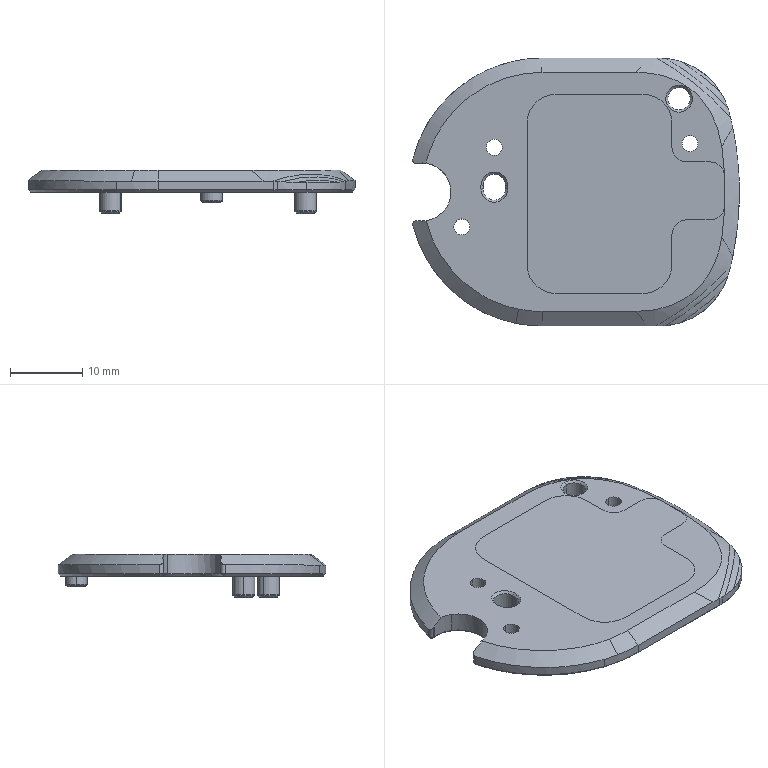NC program | NX | posted with a generic post | part box 45.101 x 36.973 x 6 mm
Lines 2609 to 3161 of 3161:
(PLANAR_MILL , TOOL : D6A45)
N5180 T01 M6
N5182 G54
N5184 G17 G0 G90 X-15.758 Y-4.63 S9500 M3
N5186 G43 Z30. H1
N5188 Z2.
N5190 G94 G1 X-15.888 Z1.965 F1250.
N5192 X-15.974 Y-4.716 Z1.932
N5194 Y-4.943 Z1.871
N5196 X-15.888 Y-5.03 Z1.839
N5198 X-15.661 Z1.778
N5200 X-15.574 Y-4.943 Z1.745
N5202 Y-4.716 Z1.684
N5204 X-15.661 Y-4.63 Z1.651
N5206 X-15.888 Z1.591
N5208 X-15.974 Y-4.716 Z1.558
N5210 Y-4.943 Z1.497
N5212 X-15.888 Y-5.03 Z1.464
N5214 X-15.661 Z1.403
N5216 X-15.574 Y-4.943 Z1.371
N5218 Y-4.716 Z1.31
N5220 X-15.661 Y-4.63 Z1.277
N5222 X-15.888 Z1.216
N5224 X-15.974 Y-4.716 Z1.183
N5226 Y-4.943 Z1.123
N5228 X-15.888 Y-5.03 Z1.09
N5230 X-15.661 Z1.029
N5232 X-15.574 Y-4.943 Z0.996
N5234 Y-4.716 Z0.935
N5236 X-15.661 Y-4.63 Z0.903
N5238 X-15.888 Z0.842
N5240 X-15.974 Y-4.716 Z0.809
N5242 Y-4.943 Z0.748
N5244 X-15.888 Y-5.03 Z0.715
N5246 X-15.661 Z0.654
N5248 X-15.574 Y-4.943 Z0.622
N5250 Y-4.716 Z0.561
N5252 X-15.661 Y-4.63 Z0.528
N5254 X-15.888 Z0.467
N5256 X-15.974 Y-4.716 Z0.434
N5258 Y-4.943 Z0.374
N5260 X-15.888 Y-5.03 Z0.341
N5262 X-15.661 Z0.28
N5264 X-15.574 Y-4.943 Z0.247
N5266 Y-4.716 Z0.186
N5268 X-15.661 Y-4.63 Z0.154
N5270 X-15.888 Z0.093
N5272 X-15.974 Y-4.716 Z0.06
N5274 Y-4.943 Z-0.001
N5276 X-15.888 Y-5.03 Z-0.034
N5278 X-15.661 Z-0.094
N5280 X-15.574 Y-4.943 Z-0.127
N5282 Y-4.716 Z-0.188
N5284 X-15.661 Y-4.63 Z-0.221
N5286 X-15.888 Z-0.282
N5288 X-15.974 Y-4.716 Z-0.314
N5290 Y-4.943 Z-0.375
N5292 X-15.888 Y-5.03 Z-0.408
N5294 X-15.661 Z-0.469
N5296 X-15.574 Y-4.943 Z-0.502
N5298 Y-4.716 Z-0.563
N5300 X-15.661 Y-4.63 Z-0.595
N5302 X-15.888 Z-0.656
N5304 X-15.974 Y-4.716 Z-0.689
N5306 Y-4.943 Z-0.75
N5308 X-15.888 Y-5.03 Z-0.783
N5310 X-15.661 Z-0.843
N5312 X-15.574 Y-4.943 Z-0.876
N5314 Y-4.716 Z-0.937
N5316 X-15.661 Y-4.63 Z-0.97
N5318 X-15.774 Z-1.
N5320 G3 X-15.974 Y-4.83 R0.2
N5322 X-15.774 Y-4.63 R-0.2
N5324 X-15.83 Y-4.839 R0.5
N5326 G1 Z2.
N5328 G0 Z30.
N5330 X-11.258 Y6.37
N5332 Z2.
N5334 G1 X-11.388 Z1.965
N5336 X-11.474 Y6.284 Z1.932
N5338 Y6.057 Z1.871
N5340 X-11.388 Y5.97 Z1.839
N5342 X-11.161 Z1.778
N5344 X-11.074 Y6.057 Z1.745
N5346 Y6.284 Z1.684
N5348 X-11.161 Y6.37 Z1.651
N5350 X-11.388 Z1.591
N5352 X-11.474 Y6.284 Z1.558
N5354 Y6.057 Z1.497
N5356 X-11.388 Y5.97 Z1.464
N5358 X-11.161 Z1.403
N5360 X-11.074 Y6.057 Z1.371
N5362 Y6.284 Z1.31
N5364 X-11.161 Y6.37 Z1.277
N5366 X-11.388 Z1.216
N5368 X-11.474 Y6.284 Z1.183
N5370 Y6.057 Z1.123
N5372 X-11.388 Y5.97 Z1.09
N5374 X-11.161 Z1.029
N5376 X-11.074 Y6.057 Z0.996
N5378 Y6.284 Z0.935
N5380 X-11.161 Y6.37 Z0.903
N5382 X-11.388 Z0.842
N5384 X-11.474 Y6.284 Z0.809
N5386 Y6.057 Z0.748
N5388 X-11.388 Y5.97 Z0.715
N5390 X-11.161 Z0.654
N5392 X-11.074 Y6.057 Z0.622
N5394 Y6.284 Z0.561
N5396 X-11.161 Y6.37 Z0.528
N5398 X-11.388 Z0.467
N5400 X-11.474 Y6.284 Z0.434
N5402 Y6.057 Z0.374
N5404 X-11.388 Y5.97 Z0.341
N5406 X-11.161 Z0.28
N5408 X-11.074 Y6.057 Z0.247
N5410 Y6.284 Z0.186
N5412 X-11.161 Y6.37 Z0.154
N5414 X-11.388 Z0.093
N5416 X-11.474 Y6.284 Z0.06
N5418 Y6.057 Z-0.001
N5420 X-11.388 Y5.97 Z-0.034
N5422 X-11.161 Z-0.094
N5424 X-11.074 Y6.057 Z-0.127
N5426 Y6.284 Z-0.188
N5428 X-11.161 Y6.37 Z-0.221
N5430 X-11.388 Z-0.282
N5432 X-11.474 Y6.284 Z-0.314
N5434 Y6.057 Z-0.375
N5436 X-11.388 Y5.97 Z-0.408
N5438 X-11.161 Z-0.469
N5440 X-11.074 Y6.057 Z-0.502
N5442 Y6.284 Z-0.563
N5444 X-11.161 Y6.37 Z-0.595
N5446 X-11.388 Z-0.656
N5448 X-11.474 Y6.284 Z-0.689
N5450 Y6.057 Z-0.75
N5452 X-11.388 Y5.97 Z-0.783
N5454 X-11.161 Z-0.843
N5456 X-11.074 Y6.057 Z-0.876
N5458 Y6.284 Z-0.937
N5460 X-11.161 Y6.37 Z-0.97
N5462 X-11.274 Z-1.
N5464 G3 X-11.474 Y6.17 R0.2
N5466 X-11.274 Y6.37 R-0.2
N5468 X-11.33 Y6.161 R0.5
N5470 G1 Z2.
N5472 G0 Z30.
N5474 X15.742 Y6.87
N5476 Z2.
N5478 G1 X15.612 Z1.965
N5480 X15.526 Y6.784 Z1.932
N5482 Y6.557 Z1.871
N5484 X15.612 Y6.47 Z1.839
N5486 X15.839 Z1.778
N5488 X15.926 Y6.557 Z1.745
N5490 Y6.784 Z1.684
N5492 X15.839 Y6.87 Z1.651
N5494 X15.612 Z1.591
N5496 X15.526 Y6.784 Z1.558
N5498 Y6.557 Z1.497
N5500 X15.612 Y6.47 Z1.464
N5502 X15.839 Z1.403
N5504 X15.926 Y6.557 Z1.371
N5506 Y6.784 Z1.31
N5508 X15.839 Y6.87 Z1.277
N5510 X15.612 Z1.216
N5512 X15.526 Y6.784 Z1.183
N5514 Y6.557 Z1.123
N5516 X15.612 Y6.47 Z1.09
N5518 X15.839 Z1.029
N5520 X15.926 Y6.557 Z0.996
N5522 Y6.784 Z0.935
N5524 X15.839 Y6.87 Z0.903
N5526 X15.612 Z0.842
N5528 X15.526 Y6.784 Z0.809
N5530 Y6.557 Z0.748
N5532 X15.612 Y6.47 Z0.715
N5534 X15.839 Z0.654
N5536 X15.926 Y6.557 Z0.622
N5538 Y6.784 Z0.561
N5540 X15.839 Y6.87 Z0.528
N5542 X15.612 Z0.467
N5544 X15.526 Y6.784 Z0.434
N5546 Y6.557 Z0.374
N5548 X15.612 Y6.47 Z0.341
N5550 X15.839 Z0.28
N5552 X15.926 Y6.557 Z0.247
N5554 Y6.784 Z0.186
N5556 X15.839 Y6.87 Z0.154
N5558 X15.612 Z0.093
N5560 X15.526 Y6.784 Z0.06
N5562 Y6.557 Z-0.001
N5564 X15.612 Y6.47 Z-0.034
N5566 X15.839 Z-0.094
N5568 X15.926 Y6.557 Z-0.127
N5570 Y6.784 Z-0.188
N5572 X15.839 Y6.87 Z-0.221
N5574 X15.612 Z-0.282
N5576 X15.526 Y6.784 Z-0.314
N5578 Y6.557 Z-0.375
N5580 X15.612 Y6.47 Z-0.408
N5582 X15.839 Z-0.469
N5584 X15.926 Y6.557 Z-0.502
N5586 Y6.784 Z-0.563
N5588 X15.839 Y6.87 Z-0.595
N5590 X15.612 Z-0.656
N5592 X15.526 Y6.784 Z-0.689
N5594 Y6.557 Z-0.75
N5596 X15.612 Y6.47 Z-0.783
N5598 X15.839 Z-0.843
N5600 X15.926 Y6.557 Z-0.876
N5602 Y6.784 Z-0.937
N5604 X15.839 Y6.87 Z-0.97
N5606 X15.726 Z-1.
N5608 G3 X15.526 Y6.67 R0.2
N5610 X15.726 Y6.87 R-0.2
N5612 X15.67 Y6.661 R0.5
N5614 G1 Z2.
N5616 G0 Z30.
(PLANAR_MILL_COPY , TOOL : D6A45)
N5618 X-11.154 Y-0.43
N5620 Z2.
N5622 G1 X-11.046 Z1.971
N5624 X-10.652 Y-0.202 Z1.849
N5626 X-10.424 Y0.192 Z1.727
N5628 Y1.148 Z1.471
N5630 X-10.652 Y1.542 Z1.349
N5632 X-11.046 Y1.77 Z1.227
N5634 X-11.502 Z1.105
N5636 X-11.896 Y1.542 Z0.983
N5638 X-12.124 Y1.148 Z0.86
N5640 Y0.192 Z0.604
N5642 X-11.896 Y-0.202 Z0.482
N5644 X-11.502 Y-0.43 Z0.36
N5646 X-11.046 Z0.238
N5648 X-10.652 Y-0.202 Z0.116
N5650 X-10.424 Y0.192 Z-0.006
N5652 Y1.148 Z-0.262
N5654 X-10.652 Y1.542 Z-0.384
N5656 X-11.046 Y1.77 Z-0.506
N5658 X-11.502 Z-0.628
N5660 X-11.896 Y1.542 Z-0.75
N5662 X-12.124 Y1.148 Z-0.872
N5664 Y0.67 Z-1.
N5666 Y0.42
N5668 G3 X-11.274 Y-0.43 R0.85
N5670 X-10.424 Y0.42 R0.85
N5672 G1 Y0.92
N5674 G3 X-11.274 Y1.77 R0.85
N5676 X-12.124 Y0.92 R0.85
N5678 G1 Y0.67
N5680 G3 X-11.767 Y-0.096 R1.
N5682 G1 Z2.
N5684 G0 Z30.
N5686 X14.485 Y13.702
N5688 Z2.
N5690 G1 X13.998 Y13.72 Z1.868
N5692 X13.604 Y13.492 Z1.746
N5694 X13.376 Y13.098 Z1.624
N5696 Y12.642 Z1.502
N5698 X13.604 Y12.248 Z1.38
N5700 X13.998 Y12.02 Z1.258
N5702 X14.454 Z1.136
N5704 X14.848 Y12.248 Z1.014
N5706 X15.076 Y12.642 Z0.892
N5708 Y13.098 Z0.77
N5710 X14.848 Y13.492 Z0.648
N5712 X14.454 Y13.72 Z0.526
N5714 X13.998 Z0.403
N5716 X13.604 Y13.492 Z0.281
N5718 X13.376 Y13.098 Z0.159
N5720 Y12.642 Z0.037
N5722 X13.604 Y12.248 Z-0.085
N5724 X13.998 Y12.02 Z-0.207
N5726 X14.454 Z-0.329
N5728 X14.848 Y12.248 Z-0.451
N5730 X15.076 Y12.642 Z-0.573
N5732 Y13.098 Z-0.695
N5734 X14.848 Y13.492 Z-0.817
N5736 X14.454 Y13.72 Z-0.939
N5738 X14.226 Z-1.
N5740 G3 X13.376 Y12.87 R0.85
N5742 X14.226 Y13.72 R-0.85
N5744 X13.843 Y13.541 R0.5
N5746 G1 Z2.
N5748 G0 Z30.
N5750 M5
(刀补 , TOOL : D2)
N5752 T17 M6
N5754 G54
N5756 G17 G0 G90 X-11.374 Y0.823 S9500 M3
N5758 G43 Z30. H17
N5760 Z0.
N5762 G94 G1 Z-1. F1000.
N5764 G41 X-11.703 D17
N5766 X-11.75 Y0.785
N5768 X-11.775 Y0.73
N5770 X-11.774 Y0.67
N5772 Y0.42
N5774 G3 X-11.274 Y-0.08 R0.5
N5776 X-10.774 Y0.42 R0.5
N5778 G1 Y0.92
N5780 G3 X-11.274 Y1.42 R0.5
N5782 X-11.774 Y0.92 R0.5
N5784 G1 Y0.67
N5786 Y0.476 Z-1.063
N5788 X-11.766 Y0.386 Z-1.092
N5790 X-11.757 Y0.323 Z-1.113
N5792 X-11.748 Y0.286 Z-1.125
N5794 X-11.72 Y0.206 Z-1.152
N5796 X-11.686 Y0.153 Z-1.173
N5798 X-11.663 Y0.115 Z-1.188
N5800 X-11.614 Y0.065 Z-1.21
N5802 X-11.59 Y0.041 Z-1.222
N5804 X-11.567 Y0.024 Z-1.231
N5806 X-11.518 Y-0.008 Z-1.25
N5808 X-11.45 Y-0.039 Z-1.275
N5810 X-11.39 Y-0.06 Z-1.295
N5812 X-11.338 Y-0.067 Z-1.313
N5814 X-11.251 Y-0.072 Z-1.341
N5816 X-11.189 Y-0.065 Z-1.361
N5818 X-11.148 Y-0.056 Z-1.375
N5820 X-11.072 Y-0.03 Z-1.401
N5822 X-11.037 Y-0.011 Z-1.414
N5824 X-10.977 Y0.027 Z-1.438
N5826 X-10.922 Y0.076 Z-1.462
N5828 X-10.88 Y0.123 Z-1.482
N5830 X-10.852 Y0.17 Z-1.5
N5832 X-10.818 Y0.235 Z-1.524
N5834 X-10.798 Y0.295 Z-1.545
N5836 X-10.789 Y0.348 Z-1.563
N5838 X-10.778 Y0.444 Z-1.594
N5840 X-10.774 Y0.541 Z-1.625
N5842 Y0.735 Z-1.688
N5844 Y0.832 Z-1.719
N5846 X-10.78 Y0.929 Z-1.75
N5848 X-10.791 Y1.019 Z-1.78
N5850 X-10.803 Y1.062 Z-1.794
N5852 X-10.822 Y1.115 Z-1.813
N5854 X-10.857 Y1.181 Z-1.837
N5856 X-10.893 Y1.233 Z-1.858
N5858 X-10.93 Y1.27 Z-1.875
N5860 X-10.993 Y1.325 Z-1.902
N5862 X-11.047 Y1.358 Z-1.923
N5864 X-11.088 Y1.376 Z-1.938
N5866 X-11.18 Y1.403 Z-1.969
N5868 X-11.274 Y1.42 Z-2.
N5870 G3 X-11.774 Y0.92 R0.5
N5872 G1 Y0.67
N5874 Y0.476 Z-2.063
N5876 X-11.766 Y0.386 Z-2.092
N5878 X-11.757 Y0.323 Z-2.113
N5880 X-11.748 Y0.286 Z-2.125
N5882 X-11.72 Y0.206 Z-2.152
N5884 X-11.686 Y0.153 Z-2.173
N5886 X-11.663 Y0.115 Z-2.188
N5888 X-11.614 Y0.065 Z-2.21
N5890 X-11.59 Y0.041 Z-2.222
N5892 X-11.567 Y0.024 Z-2.231
N5894 X-11.518 Y-0.008 Z-2.25
N5896 X-11.45 Y-0.039 Z-2.275
N5898 X-11.39 Y-0.06 Z-2.295
N5900 X-11.338 Y-0.067 Z-2.313
N5902 X-11.251 Y-0.072 Z-2.341
N5904 X-11.189 Y-0.065 Z-2.361
N5906 X-11.148 Y-0.056 Z-2.375
N5908 X-11.072 Y-0.03 Z-2.401
N5910 X-11.037 Y-0.011 Z-2.414
N5912 X-10.977 Y0.027 Z-2.438
N5914 X-10.922 Y0.076 Z-2.462
N5916 X-10.88 Y0.123 Z-2.482
N5918 X-10.852 Y0.17 Z-2.5
N5920 X-10.818 Y0.235 Z-2.524
N5922 X-10.798 Y0.295 Z-2.545
N5924 X-10.789 Y0.348 Z-2.563
N5926 X-10.778 Y0.444 Z-2.594
N5928 X-10.774 Y0.541 Z-2.625
N5930 Y0.735 Z-2.688
N5932 Y0.832 Z-2.719
N5934 X-10.78 Y0.929 Z-2.75
N5936 X-10.791 Y1.019 Z-2.78
N5938 X-10.803 Y1.062 Z-2.794
N5940 X-10.822 Y1.115 Z-2.813
N5942 X-10.857 Y1.181 Z-2.837
N5944 X-10.893 Y1.233 Z-2.858
N5946 X-10.93 Y1.27 Z-2.875
N5948 X-10.993 Y1.325 Z-2.902
N5950 X-11.047 Y1.358 Z-2.923
N5952 X-11.088 Y1.376 Z-2.938
N5954 X-11.18 Y1.403 Z-2.969
N5956 X-11.274 Y1.42 Z-3.
N5958 G3 X-11.774 Y0.92 R0.5
N5960 G1 Y0.42
N5962 G3 X-11.274 Y-0.08 R0.5
N5964 X-10.774 Y0.42 R0.5
N5966 G1 Y0.92
N5968 G3 X-11.274 Y1.42 R0.5
N5970 G1 X-11.334 Y1.421
N5972 X-11.39 Y1.396
N5974 X-11.427 Y1.349
N5976 G40
N5978 X-11.308 Y1.014
N5980 Z-2.
N5982 G0 Z30.
N5984 X14.259 Y12.964
N5986 Z0.
N5988 G1 Z-1.
N5990 G41 X14.379 Y13.299
N5992 X14.341 Y13.346
N5994 X14.286 Y13.371
N5996 X14.226 Y13.37
N5998 G3 X13.726 Y12.87 R0.5
N6000 X14.226 Y13.37 R-0.5
N6002 G1 X14.11 Y13.35 Z-1.051
N6004 X14.037 Y13.325 Z-1.084
N6006 X13.97 Y13.289 Z-1.116
N6008 X13.915 Y13.255 Z-1.144
N6010 X13.879 Y13.217 Z-1.167
N6012 X13.821 Y13.148 Z-1.205
N6014 X13.786 Y13.095 Z-1.233
N6016 X13.771 Y13.059 Z-1.25
N6018 X13.744 Y12.975 Z-1.287
N6020 X13.736 Y12.912 Z-1.315
N6022 X13.732 Y12.87 Z-1.334
N6024 X13.739 Y12.798 Z-1.365
N6026 X13.744 Y12.762 Z-1.38
N6028 X13.753 Y12.735 Z-1.393
N6030 X13.771 Y12.682 Z-1.417
N6032 X13.806 Y12.615 Z-1.449
N6034 X13.84 Y12.561 Z-1.477
N6036 X13.879 Y12.523 Z-1.5
N6038 X13.947 Y12.466 Z-1.538
N6040 X14.001 Y12.431 Z-1.566
N6042 X14.037 Y12.415 Z-1.584
N6044 X14.12 Y12.388 Z-1.621
N6046 X14.184 Y12.38 Z-1.648
N6048 X14.226 Y12.376 Z-1.667
N6050 X14.298 Y12.383 Z-1.698
N6052 X14.334 Y12.388 Z-1.714
N6054 X14.361 Y12.397 Z-1.726
N6056 X14.414 Y12.415 Z-1.75
N6058 X14.481 Y12.45 Z-1.782
N6060 X14.535 Y12.484 Z-1.81
N6062 X14.573 Y12.523 Z-1.834
N6064 X14.63 Y12.589 Z-1.871
N6066 X14.664 Y12.643 Z-1.899
N6068 X14.681 Y12.682 Z-1.917
N6070 X14.709 Y12.775 Z-1.959
N6072 X14.726 Y12.87 Z-2.
N6074 G3 X14.226 Y13.37 R0.5
N6076 G1 X14.11 Y13.35 Z-2.051
N6078 X14.037 Y13.325 Z-2.084
N6080 X13.97 Y13.289 Z-2.116
N6082 X13.915 Y13.255 Z-2.144
N6084 X13.879 Y13.217 Z-2.167
N6086 X13.821 Y13.148 Z-2.205
N6088 X13.786 Y13.095 Z-2.233
N6090 X13.771 Y13.059 Z-2.25
N6092 X13.744 Y12.975 Z-2.287
N6094 X13.736 Y12.912 Z-2.315
N6096 X13.732 Y12.87 Z-2.334
N6098 X13.739 Y12.798 Z-2.365
N6100 X13.744 Y12.762 Z-2.38
N6102 X13.753 Y12.735 Z-2.393
N6104 X13.771 Y12.682 Z-2.417
N6106 X13.806 Y12.615 Z-2.449
N6108 X13.84 Y12.561 Z-2.477
N6110 X13.879 Y12.523 Z-2.5
N6112 X13.947 Y12.466 Z-2.538
N6114 X14.001 Y12.431 Z-2.566
N6116 X14.037 Y12.415 Z-2.584
N6118 X14.12 Y12.388 Z-2.621
N6120 X14.184 Y12.38 Z-2.648
N6122 X14.226 Y12.376 Z-2.667
N6124 X14.298 Y12.383 Z-2.698
N6126 X14.334 Y12.388 Z-2.714
N6128 X14.361 Y12.397 Z-2.726
N6130 X14.414 Y12.415 Z-2.75
N6132 X14.481 Y12.45 Z-2.782
N6134 X14.535 Y12.484 Z-2.81
N6136 X14.573 Y12.523 Z-2.834
N6138 X14.63 Y12.589 Z-2.871
N6140 X14.664 Y12.643 Z-2.899
N6142 X14.681 Y12.682 Z-2.917
N6144 X14.709 Y12.775 Z-2.959
N6146 X14.726 Y12.87 Z-3.
N6148 G3 X14.226 Y13.37 R0.5
N6150 X14.726 Y12.87 R-0.5
N6152 G1 X14.727 Y12.93
N6154 X14.701 Y12.985
N6156 X14.654 Y13.023
N6158 G40
N6160 X14.32 Y12.904
N6162 Z-2.
N6164 G0 Z30.
N6166 M5
(刀补16 , TOOL : D1.5)
N6168 T16 M6
N6170 G54
N6172 G17 G0 G90 X-15.774 Y-4.83 S9500 M3
N6174 G43 Z30. H16
N6176 Z0.5
N6178 G41 G94 G1 X-15.727 Y-4.918 F1000. D16
N6180 G3 X-15.474 Y-4.83 R0.142
N6182 X-15.474 Y-4.83 Z-0.5 I-0.3 J0.
N6184 X-15.474 Y-4.83 Z-1.5 I-0.3 J0.
N6186 X-15.474 Y-4.83 Z-2.5 I-0.3 J0.
N6188 X-16.074 Y-4.83 Z-3. I-0.3 J0.
N6190 X-15.774 Y-5.13 R0.3
N6192 X-16.074 Y-4.83 R-0.3
N6194 X-15.822 Y-4.918 R0.142
N6196 G40
N6198 G1 X-15.774 Y-4.83
N6200 G0 Z30.
N6202 X-11.274 Y6.17
N6204 Z0.5
N6206 G41 G1 X-11.227 Y6.082
N6208 G3 X-10.974 Y6.17 R0.142
N6210 X-10.974 Y6.17 Z-0.5 I-0.3 J0.
N6212 X-10.974 Y6.17 Z-1.5 I-0.3 J0.
N6214 X-10.974 Y6.17 Z-2.5 I-0.3 J0.
N6216 X-11.574 Y6.17 Z-3. I-0.3 J0.
N6218 X-11.274 Y5.87 R0.3
N6220 X-11.574 Y6.17 R-0.3
N6222 X-11.322 Y6.082 R0.142
N6224 G40
N6226 G1 X-11.274 Y6.17
N6228 G0 Z30.
N6230 X15.726 Y6.67
N6232 Z0.5
N6234 G41 G1 X15.773 Y6.582
N6236 G3 X16.026 Y6.67 R0.142
N6238 X16.026 Y6.67 Z-0.5 I-0.3 J0.
N6240 X16.026 Y6.67 Z-1.5 I-0.3 J0.
N6242 X16.026 Y6.67 Z-2.5 I-0.3 J0.
N6244 X15.426 Y6.67 Z-3. I-0.3 J0.
N6246 X15.726 Y6.37 R0.3
N6248 X15.426 Y6.67 R-0.3
N6250 X15.678 Y6.582 R0.142
N6252 G40
N6254 G1 X15.726 Y6.67
N6256 G0 Z30.
N6258 M5
N6260 M2